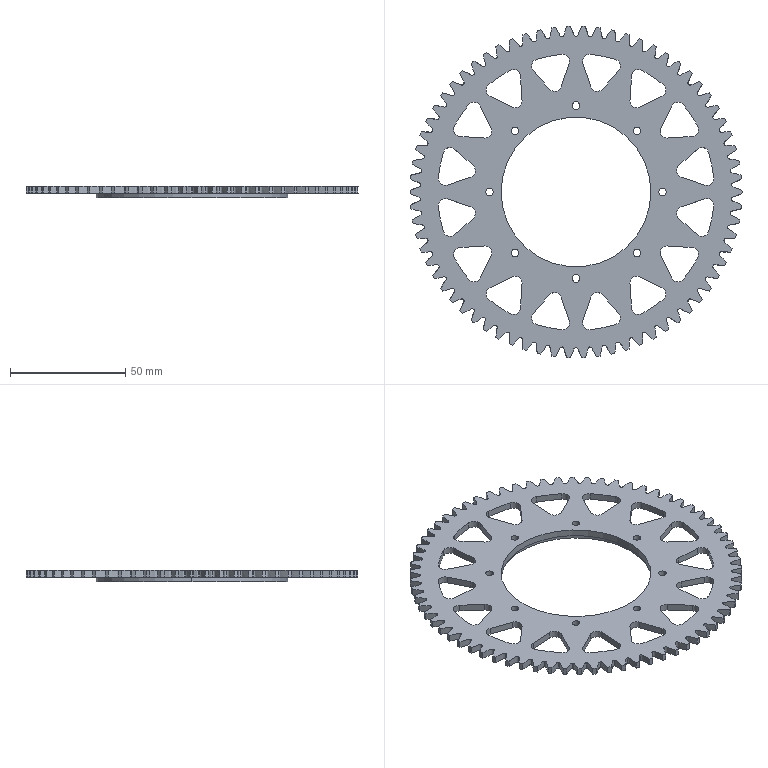Part | SolidWorks | features ICE 4, CirPattern 1, Extrusion 1, HoleWzd 1, RefAxis 1 | 1 solid | 435 faces | box 144 x 143.917 x 5 mm | volume 31123 mm3 | cylinder 243 | spline 140 | plane 36 | cone 16 | commonest cylinder face diameters 144 x71 134.999 x70 6 x64 3.3 x16 120 x16 65 x2